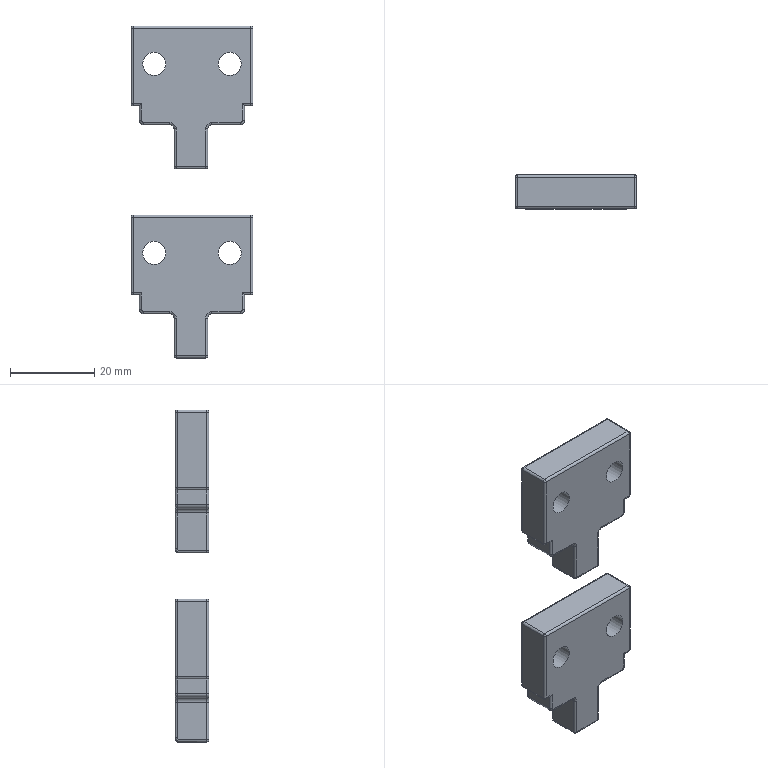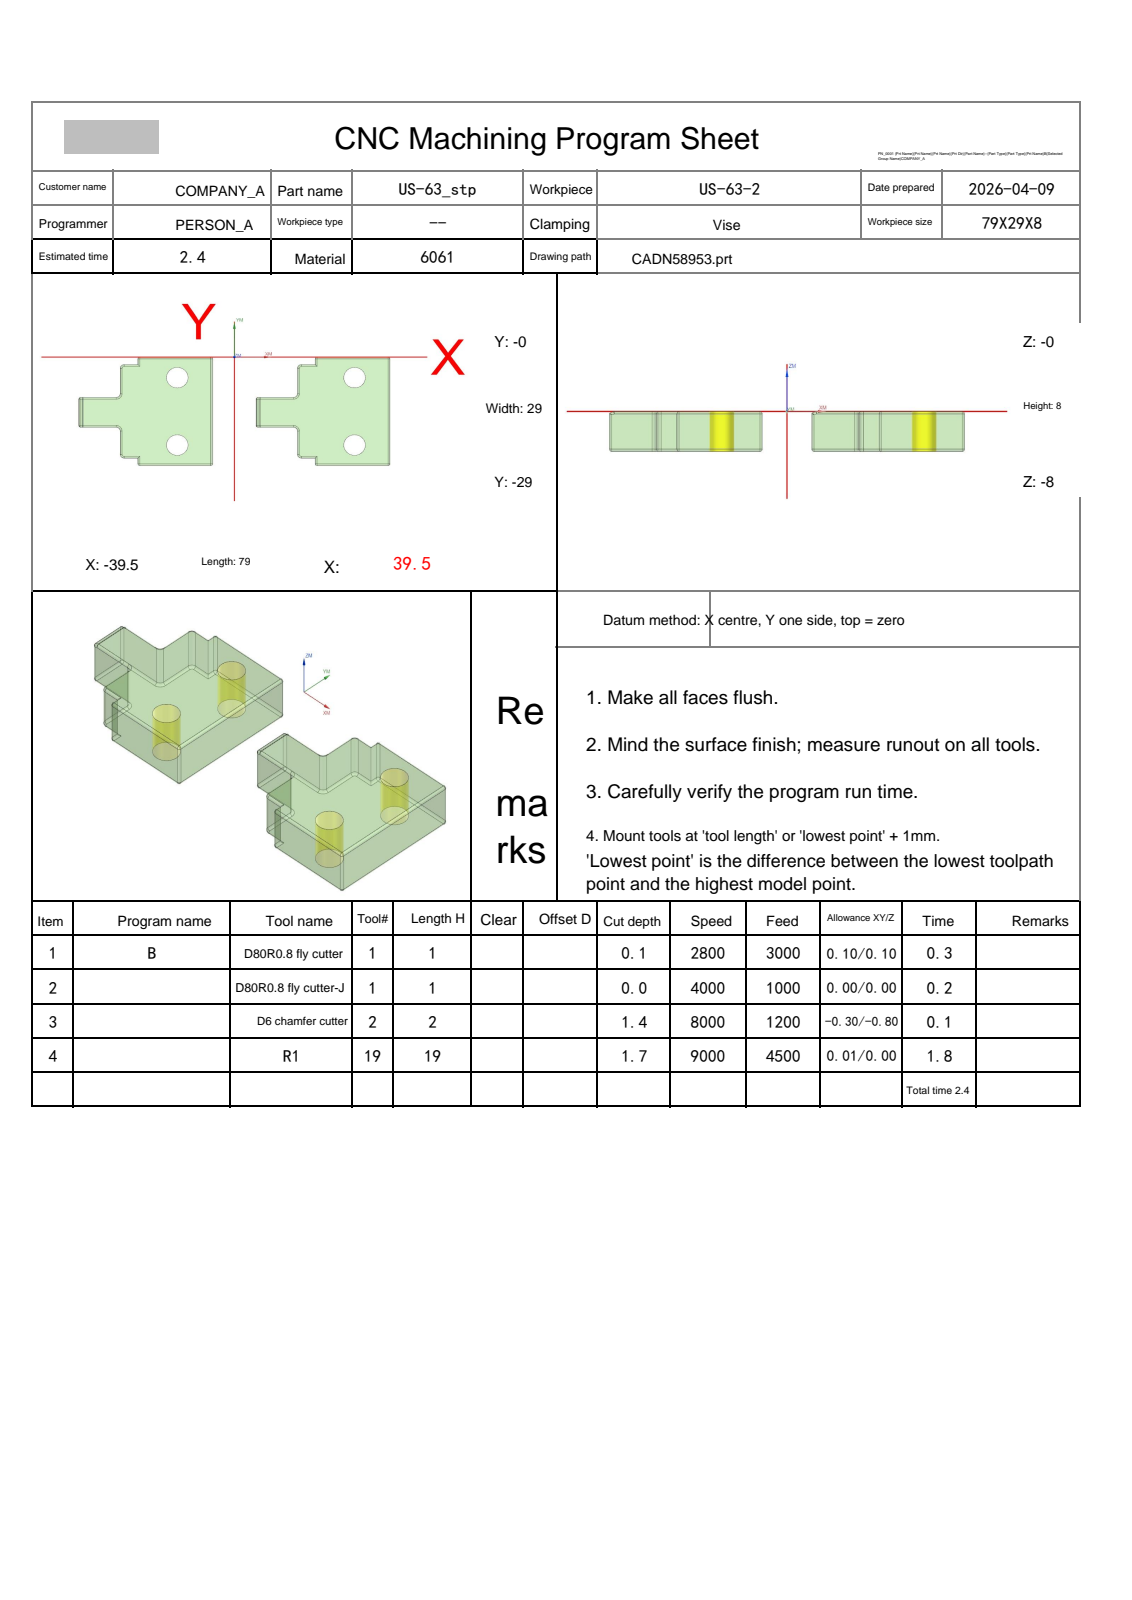NC program | NX | posted by the shop | part box 29 x 8 x 79 mm
Lines 129 to 1724 of 19198:
N4 T19 M06
(R1  D=2. R=1. H=19 ce=0.01 di=0.00)
G00 G90 G54 X16.322 Y-6.521 M03 S9000
G43 H19 Z20.
M08
Z1.5
G01 Y-2.917 Z1.311 F4500.
X16.386 Y-2.701 Z1.299
X16.517 Y-2.517 Z1.287
X16.701 Y-2.386 Z1.276
X16.917 Y-2.322 Z1.264
X20.822 Z1.059
Y-.457 Z.961
X20.87 Y-.37 Z.956
X20.957 Y-.322 Z.951
X39.043 Z.003
X39.13 Y-.37 Z-.002
X39.178 Y-.457 Z-.007
Y-.5 Z-.009
Y-28.5
G02 X39. Y-28.678 I-.178 J0.0
G01 X21.
G02 X20.822 Y-28.5 I0.0 J.178
G01 Y-26.678
X17.
G02 X16.322 Y-26. I0.0 J.678
G01 Y-19.764
G03 X15. Y-18.442 I-1.322 J0.0
G01 X6.573
G02 X6.395 Y-18.264 I0.0 J.178
G01 Y-11.264
G02 X6.573 Y-11.085 I.178 J0.0
G01 X15.
G03 X16.322 Y-9.764 I0.0 J1.322
G01 Y-3.
G02 X17. Y-2.322 I.678 J0.0
G01 X20.822
Y-.5
G02 X21. Y-.322 I.178 J0.0
G01 X39.
G02 X39.178 Y-.5 I0.0 J-.178
G01 X39.179 Y-1.5 Z-.01
X39.18 Y-2.5
X39.181 Y-3.5
X39.183 Y-4.5
X39.184 Y-5.5
X39.185 Y-6.5
X39.186 Y-7.5
X39.187 Y-8.5 Z-.011
X39.188 Y-9.5
X39.189 Y-10.5
X39.19 Y-11.5
X39.191 Y-12.5
X39.192 Y-13.5
X39.193 Y-14.5
X39.194 Y-15.5
X39.195 Y-16.5 Z-.012
X39.196 Y-17.5
X39.197 Y-18.5
X39.198 Y-19.5
X39.199 Y-20.5
X39.2 Y-21.5
X39.201 Y-22.5
X39.202 Y-23.5
X39.203 Y-24.5 Z-.013
X39.204 Y-25.5
X39.205 Y-26.5
X39.206 Y-27.5
X39.207 Y-28.5
Y-28.52
X39.203 Y-28.54
X39.199 Y-28.56
X39.191 Y-28.579
X39.184 Y-28.598
X39.172 Y-28.615
X39.161 Y-28.632
X39.146 Y-28.646
X39.132 Y-28.661
X39.115 Y-28.672
X39.098 Y-28.684
X39.079 Y-28.691
X39.06 Y-28.699
X39.04 Y-28.703
X39.02 Y-28.707
X39.
X38. Y-28.709
X37.
X36. Y-28.71 Z-.014
X35. Y-28.711
X34. Y-28.712
X33. Y-28.713
X32. Y-28.714
X31. Y-28.715
X30. Y-28.716
X29. Y-28.717 Z-.015
X28. Y-28.718
X27. Y-28.719
X26. Y-28.72
X25. Y-28.721
X24. Y-28.722
X23. Y-28.723
X22. Y-28.724
X21. Y-28.725 Z-.016
X20.978 Y-28.724
X20.956 Y-28.721
X20.935 Y-28.716
X20.914 Y-28.708
X20.894 Y-28.699
X20.875 Y-28.687
X20.857 Y-28.674
X20.841 Y-28.659
X20.826 Y-28.643
X20.813 Y-28.625
X20.801 Y-28.606
X20.792 Y-28.586
X20.784 Y-28.565
X20.779 Y-28.544
X20.775 Y-28.522
Y-28.5
X20.774 Y-27.614
X20.773 Y-26.727
X19.842 Y-26.728
X18.911 Y-26.729
X17.955 Y-26.73
X17. Y-26.731
X16.918 Y-26.726
X16.837 Y-26.713
X16.759 Y-26.69
X16.683 Y-26.659
X16.611 Y-26.619
X16.544 Y-26.572
X16.483 Y-26.517
X16.428 Y-26.456
X16.381 Y-26.389
X16.341 Y-26.317
X16.31 Y-26.241
X16.287 Y-26.163
X16.273 Y-26.082
X16.268 Y-26.
Y-25.22 Z-.017
X16.267 Y-24.441
Y-23.661
X16.266 Y-22.882
X16.265 Y-22.102
Y-21.323
X16.264 Y-20.543
X16.263 Y-19.764
X16.259 Y-19.665
X16.248 Y-19.566
X16.228 Y-19.469
X16.201 Y-19.373
X16.166 Y-19.28
X16.125 Y-19.19
X16.076 Y-19.104
X16.022 Y-19.021
X15.96 Y-18.944
X15.893 Y-18.871
X15.82 Y-18.804
X15.742 Y-18.742
X15.659 Y-18.688
X15.573 Y-18.639
X15.483 Y-18.598 Z-.018
X15.39 Y-18.563
X15.295 Y-18.537
X15.197 Y-18.517
X15.099 Y-18.506
X15. Y-18.502
X14.157 Y-18.503
X13.315
X12.472 Y-18.505
X11.629
X10.787 Y-18.506
X9.944
X9.101 Y-18.507
X8.259
X7.416 Y-18.509 Z-.019
X6.573
X6.549 Y-18.508
X6.526 Y-18.504
X6.502 Y-18.499
X6.48 Y-18.49
X6.457 Y-18.481
X6.437 Y-18.467
X6.417 Y-18.454
X6.4 Y-18.437
X6.383 Y-18.42
X6.37 Y-18.4
X6.356 Y-18.38
X6.347 Y-18.357
X6.338 Y-18.335
X6.333 Y-18.311
X6.328 Y-18.288
Y-18.264
X6.326 Y-17.389
X6.327 Y-16.514
X6.325 Y-15.639
Y-14.764
X6.324 Y-13.889
Y-13.014
X6.322 Y-12.139 Z-.02
X6.323 Y-11.264
Y-11.239
X6.327 Y-11.215
X6.332 Y-11.191
X6.342 Y-11.168
X6.351 Y-11.145
X6.365 Y-11.124
X6.379 Y-11.104
X6.396 Y-11.086
X6.413 Y-11.069
X6.434 Y-11.055
X6.455 Y-11.041
X6.477 Y-11.032
X6.5 Y-11.022
X6.524 Y-11.017
X6.549 Y-11.013
X6.573
X7.416 Y-11.011
X8.259
X9.101 Y-11.01
X9.944
X10.787 Y-11.009
X11.629
X12.472 Y-11.007
X13.315 Z-.021
X14.157 Y-11.006
X15.
X15.097 Y-11.001
X15.194 Y-10.99
X15.29 Y-10.97
X15.384 Y-10.945
X15.475 Y-10.91
X15.564 Y-10.87
X15.648 Y-10.821
X15.73 Y-10.768
X15.806 Y-10.707
X15.878 Y-10.641
X15.943 Y-10.569
X16.004 Y-10.493
X16.057 Y-10.412
X16.106 Y-10.327
X16.146 Y-10.238
X16.18 Y-10.147
X16.206 Y-10.053
X16.226 Y-9.958
X16.236 Y-9.861
X16.241 Y-9.764
X16.239 Y-8.918
Y-8.073
X16.238 Y-7.227
Y-6.382 Z-.022
X16.237 Y-5.536
Y-4.691
X16.236 Y-3.845
X16.235 Y-3.
X16.236 Y-2.957
X16.239 Y-2.914
X16.245 Y-2.872
X16.254 Y-2.83
X16.264 Y-2.788
X16.277 Y-2.747
X16.293 Y-2.707
X16.311 Y-2.668
X16.33 Y-2.63
X16.352 Y-2.593
X16.375 Y-2.557
X16.402 Y-2.523
X16.429 Y-2.49
X16.459 Y-2.459
X16.49 Y-2.429
X16.523 Y-2.402
X16.557 Y-2.375
X16.593 Y-2.352
X16.629 Y-2.33
X16.668 Y-2.31
X16.707 Y-2.292
X16.747 Y-2.277
X16.788 Y-2.264
X16.83 Y-2.254
X16.872 Y-2.245
X16.914 Y-2.239
X16.957 Y-2.235
X17. Y-2.234
X17.955 Y-2.233
X18.911
X19.821 Y-2.232
X20.731 Y-2.231 Z-.023
X20.73 Y-1.365
Y-.5
X20.731 Y-.473
X20.735 Y-.447
X20.741 Y-.421
X20.75 Y-.397
X20.761 Y-.372
X20.775 Y-.35
X20.791 Y-.328
X20.809 Y-.309
X20.828 Y-.291
X20.85 Y-.275
X20.872 Y-.261
X20.897 Y-.25
X20.921 Y-.241
X20.947 Y-.235
X20.973 Y-.23
X21.
X22. Y-.229
X23. Y-.228
X24. Y-.227
X25.
X26. Y-.226 Z-.024
X27. Y-.225
X28. Y-.224
X29. Y-.223
X30.
X31. Y-.222
X32. Y-.221
X33. Y-.22
X34. Z-.025
X35. Y-.219
X36. Y-.218
X37. Y-.217
X38.
X39. Y-.216
X39.028 Y-.217
X39.055 Y-.222
X39.082 Y-.228
X39.109 Y-.238
X39.134 Y-.249
X39.158 Y-.264
X39.18 Y-.28
X39.201 Y-.299
X39.22 Y-.32
X39.236 Y-.342
X39.251 Y-.366
X39.262 Y-.391
X39.272 Y-.417
X39.279 Y-.445
X39.283 Y-.472
X39.284 Y-.5
X39.285 Y-1.5 Z-.026
X39.286 Y-2.5
X39.287 Y-3.5
X39.288 Y-4.5
X39.289 Y-5.5
X39.29 Y-6.5
X39.291 Y-7.5 Z-.027
X39.292 Y-8.5
X39.293 Y-9.5
X39.294 Y-10.5
X39.295 Y-11.5
X39.296 Y-12.5 Z-.028
X39.297 Y-13.5
Y-14.5
X39.298 Y-15.5
X39.299 Y-16.5
X39.3 Y-17.5
X39.301 Y-18.5 Z-.029
X39.302 Y-19.5
X39.303 Y-20.5
X39.304 Y-21.5
X39.305 Y-22.5
X39.306 Y-23.5 Z-.03
Y-24.5
X39.308 Y-25.5
Y-26.5
X39.309 Y-27.5
X39.31 Y-28.5 Z-.031
X39.307 Y-28.549
X39.295 Y-28.596
X39.277 Y-28.641
X39.251 Y-28.682
X39.22 Y-28.72
X39.182 Y-28.751
X39.141 Y-28.777
X39.096 Y-28.795
X39.049 Y-28.807
X39. Y-28.81
X38. Y-28.812
X37.
X36. Y-28.813
X35. Y-28.814
X34. Y-28.815 Z-.032
X33. Y-28.816
X32. Y-28.817
X31. Y-28.818
X30. Y-28.819
X29. Y-28.82
X28. Y-28.821 Z-.033
X27.
X26. Y-28.822
X25. Y-28.823
X24. Y-28.824
X23. Y-28.825 Z-.034
X22. Y-28.826
X21. Y-28.827
X20.949 Y-28.823
X20.899 Y-28.811
X20.851 Y-28.792
X20.808 Y-28.765
X20.769 Y-28.731
X20.735 Y-28.692
X20.708 Y-28.649
X20.689 Y-28.601
X20.677 Y-28.551
X20.673 Y-28.5
X20.672 Y-27.664
X20.671 Y-26.829
X19.764 Y-26.83 Z-.035
X18.858
X17.929 Y-26.831
X17. Y-26.832
X16.953 Y-26.831
X16.907 Y-26.827
X16.861 Y-26.821
X16.815 Y-26.811
X16.77 Y-26.8
X16.725 Y-26.786
X16.681 Y-26.769
X16.639 Y-26.75
X16.597 Y-26.729
X16.557 Y-26.705
X16.518 Y-26.679
X16.481 Y-26.651
X16.445 Y-26.621
X16.411 Y-26.589
X16.379 Y-26.555
X16.349 Y-26.519
X16.321 Y-26.482
X16.295 Y-26.443
X16.271 Y-26.403
X16.25 Y-26.361
X16.23 Y-26.319
X16.214 Y-26.275
X16.199 Y-26.231
X16.188 Y-26.185
X16.179 Y-26.14
X16.172 Y-26.093
X16.168 Y-26.047
X16.167 Y-26.
X16.166 Y-25.22
X16.165 Y-24.441 Z-.036
Y-23.661
X16.164 Y-22.882
Y-22.102
X16.163 Y-21.323
Y-20.543
X16.162 Y-19.764
X16.157 Y-19.662
X16.144 Y-19.562
X16.122 Y-19.463
X16.091 Y-19.366 Z-.037
X16.052 Y-19.273
X16.006 Y-19.183
X15.951 Y-19.098
X15.889 Y-19.017
X15.821 Y-18.943
X15.746 Y-18.874
X15.666 Y-18.813
X15.58 Y-18.758
X15.49 Y-18.712
X15.397 Y-18.673
X15.3 Y-18.643
X15.202 Y-18.621
X15.101 Y-18.608
X15. Y-18.603
X14.157 Y-18.604
X13.315 Y-18.605
X12.472 Y-18.606
X11.629
X10.787 Y-18.607 Z-.038
X9.944
X9.101 Y-18.608
X8.259 Y-18.609
X7.416 Y-18.61
X6.573
X6.519 Y-18.606
X6.466 Y-18.593
X6.416 Y-18.573
X6.37 Y-18.544
X6.328 Y-18.509
X6.293 Y-18.467
X6.264 Y-18.421
X6.243 Y-18.371
X6.231 Y-18.318
X6.227 Y-18.264
X6.226 Y-17.389 Z-.039
X6.225 Y-16.514
X6.224 Y-15.639
Y-14.764
X6.223 Y-13.889
X6.222 Y-13.014
X6.221 Y-12.139 Z-.04
Y-11.264
X6.225 Y-11.208
X6.238 Y-11.155
X6.259 Y-11.103
X6.288 Y-11.057
X6.324 Y-11.014
X6.366 Y-10.979
X6.413 Y-10.949
X6.464 Y-10.928
X6.518 Y-10.915
X6.573 Y-10.911
X7.416 Y-10.91
X8.259
X9.101 Y-10.909
X9.944 Y-10.908
X10.787 Y-10.907 Z-.041
X11.629
X12.472 Y-10.906
X13.315
X14.157 Y-10.905
X15.
X15.099 Y-10.899
X15.198 Y-10.887
X15.295 Y-10.865
X15.39 Y-10.835
X15.482 Y-10.797
X15.57 Y-10.751 Z-.042
X15.654 Y-10.697
X15.733 Y-10.637
X15.806 Y-10.569
X15.873 Y-10.497
X15.933 Y-10.417
X15.987 Y-10.334
X16.032 Y-10.245
X16.071 Y-10.153
X16.1 Y-10.058
X16.122 Y-9.962
X16.135 Y-9.863
X16.14 Y-9.764
X16.139 Y-8.918
X16.138 Y-8.073
X16.137 Y-7.227
Y-6.382
X16.136 Y-5.536 Z-.043
Y-4.691
X16.135 Y-3.845
X16.134 Y-3.
X16.135 Y-2.951
X16.14 Y-2.903
X16.146 Y-2.855
X16.156 Y-2.807
X16.167 Y-2.76
X16.183 Y-2.714
X16.199 Y-2.668
X16.22 Y-2.624
X16.241 Y-2.581
X16.267 Y-2.539
X16.293 Y-2.498
X16.323 Y-2.46
X16.354 Y-2.422
X16.387 Y-2.387
X16.422 Y-2.354
X16.46 Y-2.323
X16.498 Y-2.293
X16.539 Y-2.266
X16.581 Y-2.241
X16.624 Y-2.219
X16.668 Y-2.199
X16.714 Y-2.182
X16.76 Y-2.167
X16.807 Y-2.155
X16.855 Y-2.145
X16.903 Y-2.139
X16.951 Y-2.134
X17. Y-2.133
X17.929 Y-2.132
X18.858 Z-.044
X19.744 Y-2.131
X20.63 Y-2.13
Y-1.315
X20.629 Y-.5
X20.63 Y-.471
X20.633 Y-.442
X20.639 Y-.413
X20.647 Y-.385
X20.657 Y-.358
X20.669 Y-.331
X20.683 Y-.306
X20.7 Y-.282
X20.718 Y-.259
X20.737 Y-.237
X20.759 Y-.218
X20.782 Y-.2
X20.831 Y-.169
X20.885 Y-.147
X20.942 Y-.133
X21. Y-.129
X22. Y-.128 Z-.045
X23. Y-.127
X24. Y-.126
X25.
X26. Y-.125
X27. Y-.124
X28. Y-.123 Z-.046
X29. Y-.122
X30.
X31. Y-.121
X32. Y-.12
X33. Y-.119 Z-.047
X34.
X35. Y-.118
X36. Y-.117
X37. Y-.116
X38.
X39. Y-.115 Z-.048
X39.06 Y-.12
X39.119 Y-.134
X39.175 Y-.157
X39.226 Y-.188
X39.272 Y-.228
X39.312 Y-.274
X39.343 Y-.325
X39.366 Y-.381
X39.381 Y-.44
X39.386 Y-.5
Y-1.5
X39.387 Y-2.5
X39.388 Y-3.5
X39.389 Y-4.5 Z-.049
X39.39 Y-5.5
X39.391 Y-6.5
X39.392 Y-7.5
Y-8.5 Z-.05
X39.393 Y-9.5
X39.394 Y-10.5
X39.395 Y-11.5
X39.396 Y-12.5 Z-.051
X39.397 Y-13.5
Y-14.5
X39.398 Y-15.5
X39.399 Y-16.5
X39.4 Y-17.5 Z-.052
X39.401 Y-18.5
X39.402 Y-19.5
Y-20.5
X39.403 Y-21.5 Z-.053
X39.404 Y-22.5
X39.405 Y-23.5
X39.406 Y-24.5
X39.407 Y-25.5 Z-.054
Y-26.5
X39.408 Y-27.5
X39.409 Y-28.5
X39.408 Y-28.532
X39.404 Y-28.564
X39.398 Y-28.596
X39.389 Y-28.626
X39.379 Y-28.657
X39.364 Y-28.686
X39.349 Y-28.714
X39.331 Y-28.74
X39.312 Y-28.766
X39.289 Y-28.789
X39.266 Y-28.812
X39.241 Y-28.831
X39.214 Y-28.849
X39.186 Y-28.865
X39.157 Y-28.879
X39.126 Y-28.889
X39.096 Y-28.899
X39.064 Y-28.904
X39.032 Y-28.909
X39.
X38. Y-28.911 Z-.055
X37.
X36. Y-28.912
X35. Y-28.913
X34. Y-28.914 Z-.056
X33.
X32. Y-28.915
X31. Y-28.916
X30. Y-28.917
X29. Y-28.918 Z-.057
X28. Y-28.919
X27.
X26. Y-28.92
X25. Y-28.921 Z-.058
X24. Y-28.922
X23. Y-28.923
X22.
X21. Y-28.924 Z-.059
X20.967 Y-28.923
X20.934 Y-28.919
X20.901 Y-28.913
X20.869 Y-28.904
X20.837 Y-28.893
X20.807 Y-28.878
X20.778 Y-28.862
X20.75 Y-28.844
X20.724 Y-28.823
X20.7 Y-28.8
X20.677 Y-28.776
X20.656 Y-28.75
X20.638 Y-28.722
X20.621 Y-28.693
X20.607 Y-28.663
X20.596 Y-28.631
X20.587 Y-28.599
X20.58 Y-28.566
X20.576 Y-28.533
X20.575 Y-28.5
X20.574 Y-27.713
X20.573 Y-26.927
X19.69
X18.807 Y-26.928
X17.904 Z-.06
X17. Y-26.929
X16.909 Y-26.925
X16.819 Y-26.912
X16.73 Y-26.889
X16.644 Y-26.859
X16.562 Y-26.82
X16.483 Y-26.773
X16.41 Y-26.719
X16.342 Y-26.658
X16.281 Y-26.59
X16.227 Y-26.517
X16.18 Y-26.438
X16.141 Y-26.356
X16.11 Y-26.27
X16.088 Y-26.181
X16.074 Y-26.091
X16.07 Y-26.
X16.069 Y-25.22
X16.068 Y-24.441 Z-.061
Y-23.661
X16.067 Y-22.882
Y-22.102
X16.066 Y-21.323
Y-20.543
X16.065 Y-19.764 Z-.062
X16.06 Y-19.671
X16.048 Y-19.579
X16.028 Y-19.488
X16. Y-19.4
X15.965 Y-19.314
X15.922 Y-19.232
X15.872 Y-19.153
X15.815 Y-19.08
X15.752 Y-19.011
X15.684 Y-18.949
X15.61 Y-18.892
X15.532 Y-18.842
X15.45 Y-18.8
X15.364 Y-18.764
X15.275 Y-18.736
X15.185 Y-18.716
X15.093 Y-18.704
X15. Y-18.7
X14.157 Y-18.701
X13.315 Y-18.702
X12.472 Z-.063
X11.629 Y-18.703
X10.787 Y-18.704
X9.944
X9.101 Y-18.705
X8.259 Z-.064
X7.416 Y-18.706
X6.573
X6.539
X6.504 Y-18.701
X6.47 Y-18.695
X6.437 Y-18.685
X6.404 Y-18.673
X6.372 Y-18.658
X6.342 Y-18.642
X6.313 Y-18.622
X6.285 Y-18.601
X6.26 Y-18.577
X6.236 Y-18.552
X6.215 Y-18.524
X6.188 Y-18.484
X6.167 Y-18.44
X6.157 Y-18.418
X6.15 Y-18.395
X6.136 Y-18.337
X6.13 Y-18.276
X6.129 Y-17.395
X6.128 Y-16.514 Z-.065
X6.124 Y-11.311 Z-.066
Y-11.282
Y-11.253
X6.13 Y-11.192
X6.144 Y-11.134
X6.152 Y-11.109
X6.161 Y-11.085
X6.183 Y-11.041
X6.21 Y-11.
X6.232 Y-10.972
X6.256 Y-10.946
X6.282 Y-10.922
X6.31 Y-10.901
X6.339 Y-10.881
X6.37 Y-10.864
X6.401 Y-10.848
X6.435 Y-10.837
X6.468 Y-10.827
X6.503 Y-10.82
X6.538 Y-10.816
X6.573 Y-10.815
X7.416 Y-10.814
X8.259 Y-10.813
X9.101 Y-10.812
X9.944 Z-.067
X10.787 Y-10.811
X11.629
X12.472 Y-10.81
X13.315
X14.157 Y-10.809 Z-.068
X15. Y-10.808
X15.091 Y-10.804
X15.181 Y-10.792
X15.27 Y-10.772
X15.357 Y-10.745
X15.441 Y-10.71
X15.522 Y-10.668
X15.599 Y-10.619
X15.671 Y-10.564
X15.738 Y-10.502
X15.8 Y-10.435
X15.855 Y-10.362
X15.904 Y-10.286
X15.946 Y-10.205
X15.981 Y-10.121
X16.008 Y-10.034
X16.028 Y-9.945
X16.039 Y-9.855
X16.044 Y-9.764
X16.043 Y-8.918
X16.042 Y-8.073 Z-.069
X16.041 Y-7.227
Y-6.382
X16.04 Y-5.536
Y-4.691
X16.039 Y-3.845 Z-.07
Y-3.
Y-2.953
X16.043 Y-2.906
X16.048 Y-2.859
X16.057 Y-2.812
X16.067 Y-2.766
X16.079 Y-2.721
X16.094 Y-2.676
X16.111 Y-2.632
X16.13 Y-2.588
X16.151 Y-2.546
X16.175 Y-2.505
X16.2 Y-2.466
X16.227 Y-2.427
X16.256 Y-2.389
X16.287 Y-2.354
X16.32 Y-2.32
X16.354 Y-2.287
X16.389 Y-2.256
X16.426 Y-2.227
X16.465 Y-2.2
X16.505 Y-2.174
X16.546 Y-2.151
X16.588 Y-2.13
X16.632 Y-2.111
X16.676 Y-2.093
X16.721 Y-2.079
X16.766 Y-2.066
X16.812 Y-2.056
X16.859 Y-2.047
X16.906 Y-2.042
X16.953 Y-2.038
X17. Y-2.037
X17.904
X18.807 Y-2.036 Z-.071
X19.671 Y-2.035
X20.534 Y-2.034
Y-1.267
Y-.5
X20.535 Y-.463
X20.539 Y-.427
X20.546 Y-.391
X20.556 Y-.356
X20.569 Y-.321
X20.584 Y-.288
X20.602 Y-.256
X20.623 Y-.226
X20.645 Y-.197
X20.67 Y-.17
X20.697 Y-.145
X20.726 Y-.123
X20.756 Y-.102
X20.788 Y-.084
X20.821 Y-.068
X20.856 Y-.056
X20.891 Y-.046
X20.927 Y-.039
X20.963 Y-.034
X21. Y-.033
X22. Y-.032 Z-.072
X23.
X24. Y-.031
X25. Y-.03
X26. Y-.029 Z-.073
X27.
X28. Y-.028
X29. Y-.027
X30. Z-.074
X31. Y-.026
X32. Y-.025
X33. Y-.024
X34.
X35. Y-.023 Z-.075
X36. Y-.022
X37. Y-.021
X38.
X39. Y-.02 Z-.076
X39.038 Y-.021
X39.075 Y-.026
X39.112 Y-.033
X39.148 Y-.043
X39.184 Y-.056
X39.218 Y-.072
X39.251 Y-.091
X39.282 Y-.111
X39.312 Y-.135
X39.34 Y-.16
X39.365 Y-.188
X39.389 Y-.218
X39.41 Y-.249
X39.428 Y-.282
X39.444 Y-.316
X39.457 Y-.352
X39.467 Y-.388
X39.475 Y-.425
X39.479 Y-.462
X39.481 Y-.5
Y-1.5
X39.482 Y-2.5
Y-3.5
X39.483 Y-4.5 Z-.077
X39.484 Y-5.5
X39.485 Y-6.5
Y-7.5
X39.486 Y-8.5 Z-.078
Y-9.5
X39.487 Y-10.5
X39.488 Y-11.5
X39.489 Y-12.5 Z-.079
Y-13.5
X39.49 Y-14.5
X39.491 Y-15.5
Y-16.5 Z-.08
X39.492 Y-17.5
X39.493 Y-18.5
Y-19.5
X39.494 Y-20.5
X39.495 Y-21.5 Z-.081
Y-22.5
X39.496 Y-23.5
X39.497 Y-24.5
Y-25.5 Z-.082
X39.498 Y-26.5
X39.499 Y-27.5
X39.5 Y-28.5
X39.496 Y-28.565
X39.483 Y-28.629
X39.462 Y-28.691
X39.433 Y-28.75
X39.397 Y-28.805
X39.353 Y-28.853
X39.305 Y-28.897
X39.25 Y-28.933
X39.191 Y-28.962
X39.129 Y-28.983 Z-.083
X39.065 Y-28.996
X39. Y-29.
X38. Y-29.001
X37.
X36. Y-29.002
X35. Y-29.003
X34. Y-29.004 Z-.084
X33.
X32. Y-29.005
X31. Y-29.006
X30. Z-.085
X29. Y-29.007
X28. Y-29.008
X27.
X26. Y-29.009 Z-.086
X25. Y-29.01
X24.
X23. Y-29.011
X22. Y-29.012 Z-.087
X21.
X20.933 Y-29.008
X20.867 Y-28.995
X20.804 Y-28.974
X20.744 Y-28.944
X20.688 Y-28.907
X20.637 Y-28.863
X20.593 Y-28.812
X20.556 Y-28.756
X20.526 Y-28.696
X20.505 Y-28.633
X20.491 Y-28.567
X20.487 Y-28.5
Y-27.757
X20.486 Y-27.014
X19.623 Z-.088
X18.76 Y-27.015
X17.88 Y-27.016
X17.
X16.95 Y-27.015
X16.9 Y-27.012
X16.851 Y-27.006
X16.802 Y-26.997
X16.753 Y-26.986
X16.705 Y-26.973
X16.657 Y-26.957
X16.611 Y-26.939
X16.565 Y-26.919
X16.521 Y-26.897
X16.477 Y-26.872
X16.435 Y-26.845
X16.394 Y-26.817
X16.355 Y-26.786
X16.317 Y-26.754
X16.281 Y-26.719
X16.246 Y-26.683
X16.214 Y-26.645
X16.183 Y-26.606
X16.154 Y-26.565
X16.127 Y-26.523
X16.103 Y-26.479
X16.08 Y-26.435
X16.06 Y-26.389
X16.042 Y-26.343
X16.027 Y-26.295
X16.013 Y-26.247
X16.002 Y-26.198
X15.994 Y-26.149
X15.987 Y-26.1
X15.984 Y-26.05
X15.983 Y-26. Z-.089
X15.982 Y-25.22
X15.981 Y-24.441
Y-23.661
X15.98 Y-22.882
Y-22.102
X15.979 Y-21.323 Z-.09
Y-20.543
X15.978 Y-19.764
X15.974 Y-19.668
X15.959 Y-19.573
X15.932 Y-19.467
X15.904 Y-19.389
X15.855 Y-19.289
X15.813 Y-19.22
X15.746 Y-19.131
X15.691 Y-19.072
X15.608 Y-18.998
X15.543 Y-18.951
X15.447 Y-18.894
X15.374 Y-18.86
X15.268 Y-18.824
X15.191 Y-18.805
X15.096 Y-18.791
X15. Y-18.786
X14.157 Y-18.787 Z-.091
X13.315
X12.472 Y-18.788
X11.629
X10.787 Y-18.789
X9.944 Z-.092
X9.101 Y-18.79
X8.259
X7.416 Y-18.791
X6.573
X6.512 Y-18.788
X6.452 Y-18.777
X6.393 Y-18.76
X6.337 Y-18.736
X6.284 Y-18.705
X6.234 Y-18.669
X6.199 Y-18.636
X6.167 Y-18.601
X6.152 Y-18.582
X6.117 Y-18.531
X6.088 Y-18.477
X6.07 Y-18.427
X6.055 Y-18.375
X6.041 Y-18.322 Z-.093
X6.035 Y-18.267
X6.034 Y-17.396
X6.029 Y-11.311 Z-.094
Y-11.27
X6.03 Y-11.239
X6.034 Y-11.21
X6.04 Y-11.18
X6.049 Y-11.152
X6.064 Y-11.099
X6.083 Y-11.048
X6.113 Y-10.993
X6.148 Y-10.942
X6.163 Y-10.923
X6.195 Y-10.887
X6.231 Y-10.855
X6.281 Y-10.818
X6.335 Y-10.787
X6.391 Y-10.762
X6.451 Y-10.745
X6.512 Y-10.734
X6.573 Y-10.73
X7.416 Z-.095
X8.259 Y-10.729
X9.101
X9.944 Y-10.728
X10.787
X11.629 Y-10.727 Z-.096
X12.472
X13.315 Y-10.726
X14.157
X15. Y-10.725
X15.094 Y-10.72
X15.188 Y-10.707
X15.29 Y-10.68
X15.368 Y-10.652
X15.465 Y-10.605
X15.534 Y-10.563
X15.62 Y-10.498 Z-.097
X15.68 Y-10.443
X15.751 Y-10.362
X15.799 Y-10.298
X15.853 Y-10.204
X15.888 Y-10.131
X15.923 Y-10.029
X15.942 Y-9.951
X15.956 Y-9.858
X15.961 Y-9.764
X15.96 Y-8.918
Y-8.073
X15.959 Y-7.227
Y-6.382 Z-.098
X15.958 Y-5.536
Y-4.691
X15.957 Y-3.845
X15.956 Y-3.
X15.957 Y-2.949
X15.961 Y-2.898
X15.967 Y-2.847
X15.976 Y-2.796
X15.987 Y-2.746
X16.001 Y-2.697
X16.017 Y-2.648
X16.036 Y-2.601
X16.056 Y-2.554
X16.079 Y-2.508
X16.104 Y-2.463
X16.132 Y-2.42
X16.161 Y-2.378
X16.193 Y-2.338
X16.226 Y-2.299
X16.262 Y-2.262
X16.299 Y-2.226 Z-.099
X16.338 Y-2.193
X16.378 Y-2.161
X16.42 Y-2.132
X16.463 Y-2.104
X16.508 Y-2.079
X16.553 Y-2.056
X16.6 Y-2.035
X16.648 Y-2.016
X16.697 Y-2.001
X16.746 Y-1.986
X16.796 Y-1.976
X16.847 Y-1.966
X16.898 Y-1.961
X16.949 Y-1.956
X17. Y-1.955
X17.88
X18.76 Y-1.954
X19.606 Y-1.953
X20.453
Y-1.226 Z-.1
X20.452 Y-.5
X20.453 Y-.464
X20.457 Y-.428
X20.462 Y-.393
X20.471 Y-.358
X20.481 Y-.324
X20.494 Y-.29
X20.508 Y-.258
X20.526 Y-.226
X20.544 Y-.195
X20.565 Y-.166
X20.588 Y-.139
X20.613 Y-.113
X20.639 Y-.088
X20.666 Y-.065
X20.695 Y-.044
X20.726 Y-.025
X20.758 Y-.008
X20.79 Y.007
X20.824 Y.019
X20.858 Y.029
X20.893 Y.038
X20.928 Y.044
X20.964 Y.047
X21. Y.048
X22. Y.049
X23. Z-.101
X24. Y.05
X25. Y.051
X26.
X27. Y.052
X28. Z-.102
X29. Y.053
X30. Y.054
X31.
X32. Y.055 Z-.103
X33. Y.056
X34.
X35. Y.057
X36. Z-.104
X37. Y.058
X38. Y.059
X39.
X39.073 Y.055
X39.145 Y.04
X39.214 Y.017
X39.28 Y-.016
X39.341 Y-.056
X39.396 Y-.104
X39.444 Y-.159
X39.485 Y-.22
X39.517 Y-.286
X39.541 Y-.355
X39.555 Y-.427
X39.56 Y-.5
Y-1.5 Z-.105
X39.561 Y-2.5
X39.562 Y-3.5
Y-4.5
X39.563 Y-5.5 Z-.106
Y-6.5
X39.564 Y-7.5
Y-8.5
X39.565 Y-9.5 Z-.107
Y-10.5
X39.567 Y-11.5
Y-12.5
X39.568 Y-13.5 Z-.108
Y-14.5
X39.569 Y-15.5
Y-16.5
X39.57 Y-17.5
Y-18.5 Z-.109
X39.571 Y-19.5
Y-20.5
X39.572 Y-21.5
Y-22.5 Z-.11
X39.573 Y-23.5
X39.574 Y-24.5
Y-25.5
X39.575 Y-26.5 Z-.111
Y-27.5
X39.576 Y-28.5
X39.575 Y-28.538
X39.571 Y-28.575
X39.565 Y-28.612
X39.556 Y-28.649
X39.546 Y-28.685
X39.532 Y-28.72
X39.517 Y-28.755
X39.499 Y-28.788
X39.479 Y-28.82
X39.457 Y-28.851
X39.434 Y-28.88
X39.407 Y-28.907
X39.38 Y-28.934
X39.351 Y-28.957
X39.32 Y-28.979
X39.288 Y-28.999
X39.255 Y-29.017
X39.221 Y-29.032
X39.185 Y-29.046
X39.149 Y-29.057
X39.113 Y-29.066
X39.075 Y-29.071
X39.038 Y-29.076
X39.
X38. Y-29.077 Z-.112
X37. Y-29.078
X36.
X35. Y-29.079
X34.
X33. Y-29.08 Z-.113
X32.
X31. Y-29.081
X30. Y-29.082
X29. Z-.114
X28. Y-29.083
X27.
X26. Y-29.084
X25. Y-29.085 Z-.115
X24.
X23. Y-29.086
X22.
X21. Y-29.087
X20.962 Y-29.086 Z-.116
X20.923 Y-29.082
X20.885 Y-29.076
X20.848 Y-29.067
X20.811 Y-29.056
X20.775 Y-29.042
X20.74 Y-29.027
X20.706 Y-29.008
X20.674 Y-28.988
X20.643 Y-28.966
X20.613 Y-28.942
X20.585 Y-28.915
X20.558 Y-28.887
X20.534 Y-28.857
X20.512 Y-28.826
X20.491 Y-28.794
X20.473 Y-28.76
X20.457 Y-28.725
X20.444 Y-28.689
X20.433 Y-28.652
X20.424 Y-28.615
X20.418 Y-28.577
X20.414 Y-28.538
X20.413 Y-28.5
X20.412 Y-27.794
Y-27.088
X19.566 Y-27.089
X18.72
X17.86 Y-27.09 Z-.117
X17.
X16.905 Y-27.086
X16.811 Y-27.074
X16.718 Y-27.053
X16.627 Y-27.025
X16.539 Y-26.988
X16.455 Y-26.944
X16.374 Y-26.893
X16.299 Y-26.836
X16.229 Y-26.771
X16.164 Y-26.701
X16.106 Y-26.626
X16.055 Y-26.545
X16.011 Y-26.461
X15.975 Y-26.373
X15.946 Y-26.282
X15.925 Y-26.189
X15.913 Y-26.095
X15.909 Y-26.
Y-25.22
X15.908 Y-24.441 Z-.118
Y-23.661
X15.907 Y-22.882
Y-22.102
X15.906 Y-21.323
Y-20.543 Z-.119
X15.905 Y-19.764
X15.901 Y-19.675
X15.888 Y-19.587
X15.862 Y-19.488
X15.836 Y-19.417
X15.791 Y-19.324
X15.752 Y-19.261
X15.69 Y-19.178
X15.64 Y-19.124
X15.562 Y-19.055
X15.503 Y-19.011
X15.413 Y-18.959
X15.346 Y-18.928
X15.248 Y-18.894
X15.176 Y-18.876
X15.089 Y-18.863
X15. Y-18.859
X14.157
X13.315 Y-18.86
X12.472 Z-.12
X11.629 Y-18.861
X10.787
X9.944 Y-18.862
X9.101
X8.259 Y-18.863 Z-.121
X7.416
X6.573 Y-18.864
X6.508 Y-18.86
X6.443 Y-18.849
X6.379 Y-18.832
X6.318 Y-18.807
X6.26 Y-18.776
X6.206 Y-18.738
X6.188 Y-18.725
X6.172 Y-18.71
X6.142 Y-18.681
X6.114 Y-18.649
X6.068 Y-18.596
X6.026 Y-18.539
X6.008 Y-18.508
X5.992 Y-18.477
X5.98 Y-18.443
X5.969 Y-18.409
X5.958 Y-18.375
X5.948 Y-18.34
X5.942 Y-18.305
X5.939 Y-18.269
X5.938 Y-17.391
X5.934 Y-12.136 Z-.123
Y-11.258
X5.937 Y-11.222
X5.943 Y-11.186
X5.952 Y-11.151
X5.963 Y-11.116
X5.974 Y-11.082
X5.987 Y-11.049
X6.004 Y-11.017
X6.023 Y-10.986
X6.064 Y-10.928
X6.112 Y-10.876
X6.139 Y-10.843
X6.169 Y-10.814
X6.186 Y-10.799
X6.203 Y-10.786
X6.258 Y-10.748
X6.316 Y-10.716
X6.378 Y-10.691
X6.442 Y-10.673
X6.507 Y-10.662
X6.573 Y-10.659
X7.416 Y-10.658
X8.259 Z-.124
X9.101
X9.944 Y-10.657
X10.787
X11.629 Y-10.656
X12.472 Z-.125
X13.315 Y-10.655
X14.157
X15. Y-10.654
X15.087 Y-10.65
X15.174 Y-10.637
X15.269 Y-10.612
X15.341 Y-10.586
X15.431 Y-10.543
X15.495 Y-10.504
X15.574 Y-10.443
X15.63 Y-10.393
X15.696 Y-10.318
X15.74 Y-10.258
X15.791 Y-10.172
X15.822 Y-10.104
X15.855 Y-10.01
X15.873 Y-9.937
X15.885 Y-9.851
X15.89 Y-9.764
Y-8.918 Z-.126
X15.889 Y-8.073
Y-7.227
X15.888 Y-6.382
Y-5.536
X15.887 Y-4.691 Z-.127
Y-3.845
X15.886 Y-3.
X15.89 Y-2.903
X15.903 Y-2.807
X15.924 Y-2.712
X15.953 Y-2.619
X15.99 Y-2.529
X16.035 Y-2.443
X16.087 Y-2.361
X16.147 Y-2.284
X16.212 Y-2.212
X16.284 Y-2.147
X16.361 Y-2.087
X16.443 Y-2.035
X16.529 Y-1.99
X16.619 Y-1.953
X16.711 Y-1.923
X16.806 Y-1.903
X16.903 Y-1.889
X17. Y-1.885
X17.86 Z-.128
X18.72
X19.552 Y-1.884
X20.383 Y-1.883
Y-1.192
Y-.5 Z-.129
X20.384 Y-.46
X20.388 Y-.419
X20.394 Y-.38
X20.404 Y-.34
X20.415 Y-.301
X20.43 Y-.264
X20.446 Y-.227
X20.465 Y-.191
X20.486 Y-.157
X20.51 Y-.124
X20.536 Y-.093
X20.563 Y-.063
X20.593 Y-.036
X20.624 Y-.01
X20.657 Y.014
X20.691 Y.035
X20.727 Y.054
X20.764 Y.07
X20.801 Y.085
X20.84 Y.096
X20.879 Y.106
X20.919 Y.112
X20.96 Y.117
X21. Y.118
X22.
X23. Y.119
X24.
X25. Y.12 Z-.13
X26.
X27. Y.121
X28.
X29. Y.122 Z-.131
X30.
X31. Y.123
X32.
X33. Y.124 Z-.132
X34.
X35. Y.125
X36. Y.126
X37. Z-.133
X38. Y.127
X39.
X39.041 Y.126
X39.082 Y.122
X39.122 Y.115
X39.162 Y.106
X39.202 Y.094
X39.24 Y.08
X39.278 Y.063
X39.314 Y.043
X39.349 Y.022
X39.382 Y-.002
X39.414 Y-.028
X39.444 Y-.056
X39.472 Y-.086
X39.498 Y-.118
X39.522 Y-.151
X39.543 Y-.186
X39.563 Y-.222
X39.58 Y-.26
X39.594 Y-.298
X39.606 Y-.338
X39.616 Y-.378
X39.622 Y-.418
X39.627 Y-.459
X39.628 Y-.5
Y-1.5
X39.629 Y-2.5 Z-.134
Y-3.5
X39.63 Y-4.5
Y-5.5
X39.631 Y-6.5 Z-.135
Y-7.5
X39.632 Y-8.5
Y-9.5
X39.633 Y-10.5 Z-.136
Y-11.5
X39.634 Y-12.5
Y-13.5
X39.635 Y-14.5
Y-15.5 Z-.137
X39.636 Y-16.5
Y-17.5
X39.637 Y-18.5
Y-19.5 Z-.138
X39.638 Y-20.5
Y-21.5
X39.639 Y-22.5
Y-23.5 Z-.139
X39.64 Y-24.5
Y-25.5
X39.641 Y-26.5
Y-27.5 Z-.14
X39.642 Y-28.5
X39.638 Y-28.572
X39.626 Y-28.643
X39.606 Y-28.712
X39.578 Y-28.779
X39.544 Y-28.842
X39.502 Y-28.9
X39.454 Y-28.954
X39.4 Y-29.002
X39.342 Y-29.044
X39.279 Y-29.079
X39.212 Y-29.106
X39.143 Y-29.126